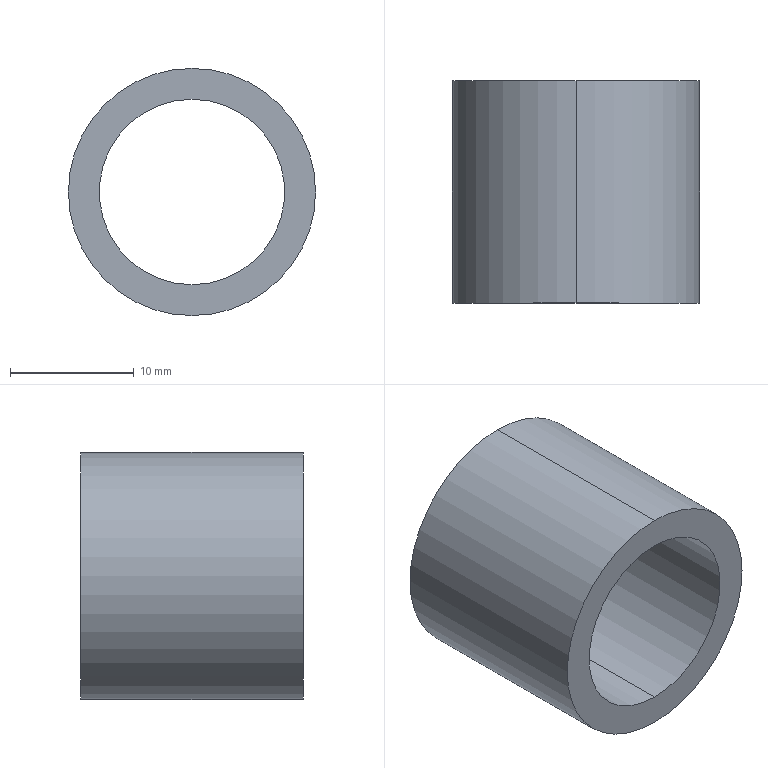Part | SolidWorks | features BaseBody 1 | 1 solid | 6 faces | box 20 x 18 x 20 mm | volume 2474 mm3 | cylinder 4 | plane 2 | commonest cylinder face diameters 15 x2 20 x2
STEP:
#1=CARTESIAN_POINT('',(0.,18.,-10.));
#2=VERTEX_POINT('',#1);
#3=CARTESIAN_POINT('',(0.,18.,10.));
#4=VERTEX_POINT('',#3);
#5=CARTESIAN_POINT('',(0.,18.,0.));
#6=DIRECTION('',(0.,-1.,0.));
#7=DIRECTION('',(0.,0.,-1.));
#8=AXIS2_PLACEMENT_3D('',#5,#6,#7);
#9=CIRCLE('',#8,10.);
#10=EDGE_CURVE('',#2,#4,#9,.T.);
#11=ORIENTED_EDGE('',*,*,#10,.T.);
#12=CARTESIAN_POINT('',(0.,0.,10.));
#13=VERTEX_POINT('',#12);
#14=CARTESIAN_POINT('',(0.,18.,10.));
#15=DIRECTION('',(0.,-1.,0.));
#16=VECTOR('',#15,1000.);
#17=LINE('',#14,#16);
#18=EDGE_CURVE('',#4,#13,#17,.T.);
#19=ORIENTED_EDGE('',*,*,#18,.T.);
#20=CARTESIAN_POINT('',(0.,0.,-10.));
#21=VERTEX_POINT('',#20);
#22=CARTESIAN_POINT('',(0.,0.,0.));
#23=DIRECTION('',(0.,1.,0.));
#24=DIRECTION('',(0.,0.,-1.));
#25=AXIS2_PLACEMENT_3D('',#22,#23,#24);
#26=CIRCLE('',#25,10.);
#27=EDGE_CURVE('',#13,#21,#26,.T.);
#28=ORIENTED_EDGE('',*,*,#27,.T.);
#29=CARTESIAN_POINT('',(0.,18.,-10.));
#30=DIRECTION('',(0.,-1.,0.));
#31=VECTOR('',#30,1000.);
#32=LINE('',#29,#31);
#33=EDGE_CURVE('',#2,#21,#32,.T.);
#34=ORIENTED_EDGE('',*,*,#33,.F.);
#35=EDGE_LOOP('',(#11,#19,#28,#34));
#36=FACE_OUTER_BOUND('',#35,.T.);
#37=CARTESIAN_POINT('',(0.,18.,0.));
#38=DIRECTION('',(0.,-1.,0.));
#39=DIRECTION('',(0.,0.,-1.));
#40=AXIS2_PLACEMENT_3D('',#37,#38,#39);
#41=CYLINDRICAL_SURFACE('',#40,10.);
#42=ADVANCED_FACE('',(#36),#41,.T.);
#43=CARTESIAN_POINT('',(0.,18.,7.5));
#44=VERTEX_POINT('',#43);
#45=CARTESIAN_POINT('',(0.,18.,-7.5));
#46=VERTEX_POINT('',#45);
#47=CARTESIAN_POINT('',(0.,18.,0.));
#48=DIRECTION('',(0.,-1.,0.));
#49=DIRECTION('',(0.,0.,-1.));
#50=AXIS2_PLACEMENT_3D('',#47,#48,#49);
#51=CIRCLE('',#50,7.5);
#52=EDGE_CURVE('',#44,#46,#51,.T.);
#53=ORIENTED_EDGE('',*,*,#52,.F.);
#54=CARTESIAN_POINT('',(0.,0.,7.5));
#55=VERTEX_POINT('',#54);
#56=CARTESIAN_POINT('',(0.,18.,7.5));
#57=DIRECTION('',(0.,-1.,0.));
#58=VECTOR('',#57,1000.);
#59=LINE('',#56,#58);
#60=EDGE_CURVE('',#44,#55,#59,.T.);
#61=ORIENTED_EDGE('',*,*,#60,.T.);
#62=CARTESIAN_POINT('',(0.,0.,-7.5));
#63=VERTEX_POINT('',#62);
#64=CARTESIAN_POINT('',(0.,0.,0.));
#65=DIRECTION('',(0.,-1.,0.));
#66=DIRECTION('',(0.,0.,-1.));
#67=AXIS2_PLACEMENT_3D('',#64,#65,#66);
#68=CIRCLE('',#67,7.5);
#69=EDGE_CURVE('',#55,#63,#68,.T.);
#70=ORIENTED_EDGE('',*,*,#69,.T.);
#71=CARTESIAN_POINT('',(0.,18.,-7.5));
#72=DIRECTION('',(0.,-1.,0.));
#73=VECTOR('',#72,1000.);
#74=LINE('',#71,#73);
#75=EDGE_CURVE('',#46,#63,#74,.T.);
#76=ORIENTED_EDGE('',*,*,#75,.F.);
#77=EDGE_LOOP('',(#53,#61,#70,#76));
#78=FACE_OUTER_BOUND('',#77,.T.);
#79=CARTESIAN_POINT('',(0.,18.,0.));
#80=DIRECTION('',(0.,-1.,0.));
#81=DIRECTION('',(0.,0.,-1.));
#82=AXIS2_PLACEMENT_3D('',#79,#80,#81);
#83=CYLINDRICAL_SURFACE('',#82,7.5);
#84=ADVANCED_FACE('',(#78),#83,.F.);
#85=ORIENTED_EDGE('',*,*,#18,.F.);
#86=CARTESIAN_POINT('',(0.,18.,0.));
#87=DIRECTION('',(0.,-1.,0.));
#88=DIRECTION('',(0.,0.,-1.));
#89=AXIS2_PLACEMENT_3D('',#86,#87,#88);
#90=CIRCLE('',#89,10.);
#91=EDGE_CURVE('',#4,#2,#90,.T.);
#92=ORIENTED_EDGE('',*,*,#91,.T.);
#93=ORIENTED_EDGE('',*,*,#33,.T.);
#94=CARTESIAN_POINT('',(0.,0.,0.));
#95=DIRECTION('',(0.,1.,0.));
#96=DIRECTION('',(0.,0.,-1.));
#97=AXIS2_PLACEMENT_3D('',#94,#95,#96);
#98=CIRCLE('',#97,10.);
#99=EDGE_CURVE('',#21,#13,#98,.T.);
#100=ORIENTED_EDGE('',*,*,#99,.T.);
#101=EDGE_LOOP('',(#85,#92,#93,#100));
#102=FACE_OUTER_BOUND('',#101,.T.);
#103=CARTESIAN_POINT('',(0.,18.,0.));
#104=DIRECTION('',(0.,-1.,0.));
#105=DIRECTION('',(0.,0.,-1.));
#106=AXIS2_PLACEMENT_3D('',#103,#104,#105);
#107=CYLINDRICAL_SURFACE('',#106,10.);
#108=ADVANCED_FACE('',(#102),#107,.T.);
#109=CARTESIAN_POINT('',(0.,0.,0.));
#110=DIRECTION('',(0.,-1.,0.));
#111=DIRECTION('',(0.,0.,-1.));
#112=AXIS2_PLACEMENT_3D('',#109,#110,#111);
#113=CIRCLE('',#112,7.5);
#114=EDGE_CURVE('',#63,#55,#113,.T.);
#115=ORIENTED_EDGE('',*,*,#114,.F.);
#116=ORIENTED_EDGE('',*,*,#69,.F.);
#117=EDGE_LOOP('',(#115,#116));
#118=FACE_BOUND('',#117,.T.);
#119=ORIENTED_EDGE('',*,*,#99,.F.);
#120=ORIENTED_EDGE('',*,*,#27,.F.);
#121=EDGE_LOOP('',(#119,#120));
#122=FACE_OUTER_BOUND('',#121,.T.);
#123=CARTESIAN_POINT('',(0.,0.,0.));
#124=DIRECTION('',(0.,1.,0.));
#125=DIRECTION('',(0.,0.,1.));
#126=AXIS2_PLACEMENT_3D('',#123,#124,#125);
#127=PLANE('',#126);
#128=ADVANCED_FACE('',(#118,#122),#127,.F.);
#129=CARTESIAN_POINT('',(0.,18.,0.));
#130=DIRECTION('',(0.,-1.,0.));
#131=DIRECTION('',(0.,0.,-1.));
#132=AXIS2_PLACEMENT_3D('',#129,#130,#131);
#133=CIRCLE('',#132,7.5);
#134=EDGE_CURVE('',#46,#44,#133,.T.);
#135=ORIENTED_EDGE('',*,*,#134,.T.);
#136=ORIENTED_EDGE('',*,*,#52,.T.);
#137=EDGE_LOOP('',(#135,#136));
#138=FACE_BOUND('',#137,.T.);
#139=ORIENTED_EDGE('',*,*,#10,.F.);
#140=ORIENTED_EDGE('',*,*,#91,.F.);
#141=EDGE_LOOP('',(#139,#140));
#142=FACE_OUTER_BOUND('',#141,.T.);
#143=CARTESIAN_POINT('',(0.,18.,0.));
#144=DIRECTION('',(0.,1.,0.));
#145=DIRECTION('',(0.,0.,1.));
#146=AXIS2_PLACEMENT_3D('',#143,#144,#145);
#147=PLANE('',#146);
#148=ADVANCED_FACE('',(#138,#142),#147,.T.);
#149=ORIENTED_EDGE('',*,*,#60,.F.);
#150=ORIENTED_EDGE('',*,*,#134,.F.);
#151=ORIENTED_EDGE('',*,*,#75,.T.);
#152=ORIENTED_EDGE('',*,*,#114,.T.);
#153=EDGE_LOOP('',(#149,#150,#151,#152));
#154=FACE_OUTER_BOUND('',#153,.T.);
#155=CARTESIAN_POINT('',(0.,18.,0.));
#156=DIRECTION('',(0.,-1.,0.));
#157=DIRECTION('',(0.,0.,-1.));
#158=AXIS2_PLACEMENT_3D('',#155,#156,#157);
#159=CYLINDRICAL_SURFACE('',#158,7.5);
#160=ADVANCED_FACE('',(#154),#159,.F.);
#161=CLOSED_SHELL('',(#42,#84,#108,#128,#148,#160));
#162=MANIFOLD_SOLID_BREP('',#161);
#163=CARTESIAN_POINT('',(0.,0.,0.));
#164=DIRECTION('',(0.,0.,1.));
#165=DIRECTION('',(1.,0.,0.));
#166=AXIS2_PLACEMENT_3D('',#163,#164,#165);
#167=(LENGTH_UNIT()NAMED_UNIT(*)SI_UNIT(.MILLI.,.METRE.));
#168=UNCERTAINTY_MEASURE_WITH_UNIT(LENGTH_MEASURE(0.00001),#167,'','');
#169=(NAMED_UNIT(*)PLANE_ANGLE_UNIT()SI_UNIT($,.RADIAN.));
#170=(NAMED_UNIT(*)SI_UNIT($,.STERADIAN.)SOLID_ANGLE_UNIT());
#171=(GEOMETRIC_REPRESENTATION_CONTEXT(3)GLOBAL_UNCERTAINTY_ASSIGNED_CONTEXT((#168))GLOBAL_UNIT_ASSIGNED_CONTEXT((#167,#169,#170))REPRESENTATION_CONTEXT('',''));
#172=ADVANCED_BREP_SHAPE_REPRESENTATION('',(#162,#166),#171);